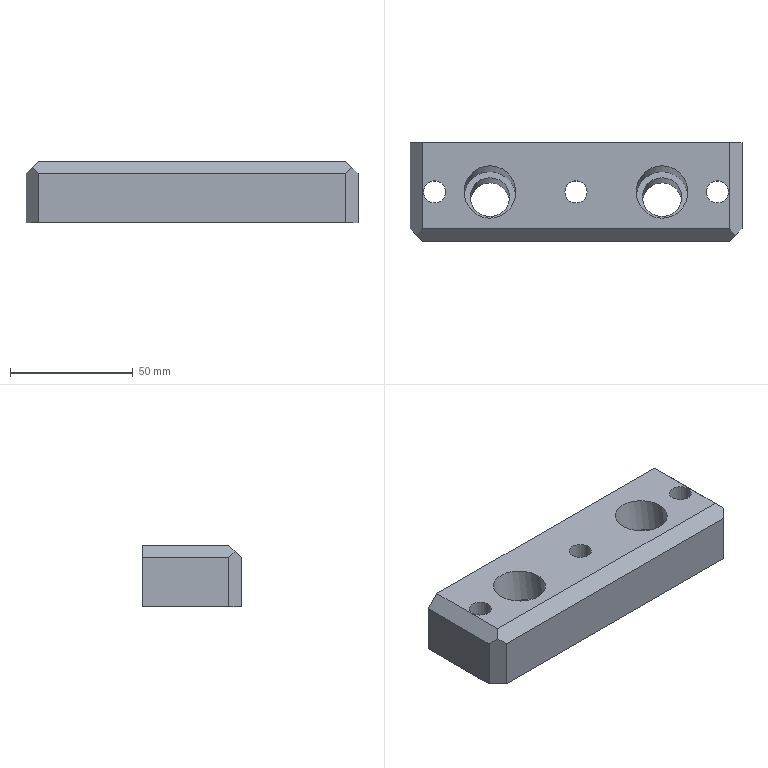Part | STEP file | P011002S004-009 | 1 solid | 26 faces | box 135 x 40 x 25 mm | volume 110970 mm3 | plane 16 | cylinder 10 | commonest cylinder face diameters 9 x3 14 x3 16 x2 21 x2